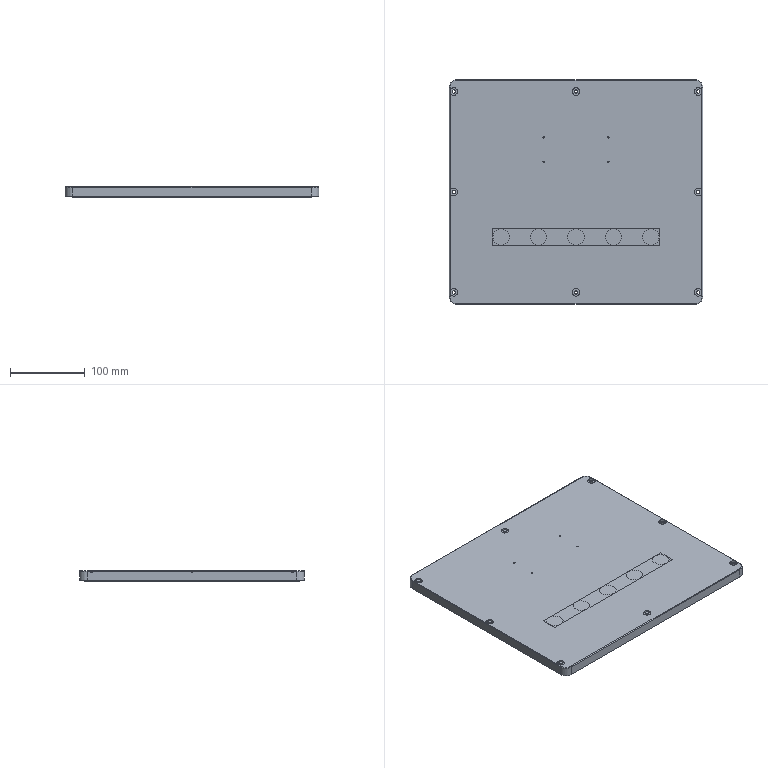NC program | NX | posted with a generic post | part box 338 x 300 x 14.5 mm
Lines 1 to 2036 of 2954, first 1954 of 2022 lines:
N10 G17 G21 G94 G90
(FLOOR_WALL , TOOL : D63)
N12 T03 M6
N14 G54
N16 G17 G0 G90 X-207. Y153.497 S6500 M3
N18 G43 Z30. H3
N20 Z3.
N22 G94 G1 Z0. F1250.
N24 X-204.
N26 X204.
N28 Y106.531
N30 X-204.
N32 Y59.565
N34 X204.
N36 Y12.599
N38 X-204.
N40 Y-34.368
N42 X204.
N44 Y-81.334
N46 X-204.
N48 Y-128.3
N50 X204.
N52 X207.
N54 Z3.
N56 G0 Z30.
N58 M5
(DRILLING_COPY_1 , TOOL : D6A45)
N60 T01 M6
N62 G54
N64 G17 G0 G90 X163. Y-134. S5000 M3
N66 G43 Z30. H1
N68 G94 G81 G98 Z-0.6 F250. R3.
N70 X100. Y-60.
N72 X163. Y0.
N74 Y134.
N76 X0.
N78 X-43. Y73.
N80 Y40.
N82 X43. Y73.
N84 Y40.
N86 X50. Y-60.
N88 X0.
N90 Y-134.
N92 X-50. Y-60.
N94 X-100.
N96 X-163. Y-134.
N98 Y0.
N100 Y134.
N102 G80
N104 G0 X-163. Y134. Z30.
N106 M5
(DRILLING_COPY_COPY , TOOL : 2.1ZT)
N108 T20 M6
N110 G54
N112 G17 G0 G90 X43. Y73. S1447 M3
N114 G43 Z30. H20
N116 G94 G83 G98 Z-7.116 F100. Q2. R3.
N118 Y40.
N120 X-43.
N122 Y73.
N124 G80
N126 G0 X-43. Y73. Z30.
N128 M5
(DRILLING_COPY_COPY_COPY , TOOL : 4.5ZT)
N130 T11 M6
N132 G54
N134 G17 G0 G90 X-163. Y134. S1447 M3
N136 G43 Z30. H11
N138 G94 G83 G98 Z-15.352 F100. Q2. R3.
N140 Y0.
N142 Y-134.
N144 X0.
N146 X163.
N148 Y0.
N150 Y134.
N152 X0.
N154 G80
N156 G0 X0. Y134. Z30.
N158 M5
(ADAPTIVE_MILLING , TOOL : D10)
N160 T04 M6
N162 G54
N164 G17 G0 G90 X-180.209 Y-0.062 S9500 M3
N166 G43 Z30. H4
N168 Z-13.5
N170 G94 G1 Z-14.5 F1000.
N172 X-179.429 Y-0.342 F3000.
N174 X-178.64 Y-0.598
N176 G3 X-177.562 Y-0.062 R1.017
N178 X-176.801 Y3.001 R8.28
N180 X-176.519 Y12.869 R111.643
N182 G1 X-176.514 Y15.119
N184 X-176.511 Y18.994
N186 X-176.51 Y32.619
N188 Y150.369
N190 Y150.494
N192 X-176.508 Y150.619
N194 G2 X-174.014 Y154.9 R5.714
N196 X-168.574 Y156.964 R12.307
N198 X-160.721 Y157.449 R56.36
N200 G1 X-159.721 Y157.46
N202 X-158.471 Y157.47
N204 X-156.846 Y157.478
N206 X-154.846 Y157.483
N208 X-151.596 Y157.487
N210 X-143.596 Y157.488
N212 X-29.346
N214 X-28.596 Y157.492
N216 X-27.471 Y157.494
N218 X-26.596
N220 X-25.846 Y157.496
N222 X-24.721
N224 X-24.346 Y157.495
N226 X-23.471 Y157.498
N228 X-22.471 Y157.496
N230 X-21.971
N232 X-21.346 Y157.497
N234 X-19.971
N236 X-19.221 Y157.496
N238 X-18.221 Y157.499
N240 X-16.971 Y157.497
N242 X-16.221 Y157.498
N244 X-15.221
N246 X-14.846 Y157.497
N248 X-13.596 Y157.5
N250 X-12.721 Y157.498
N252 X-11.471 Y157.5
N254 X-10.096 Y157.497
N256 X-9.471 Y157.499
N258 X-7.971 Y157.498
N260 X-6.971 Y157.496
N262 X-6.096 Y157.499
N264 X-5.471 Y157.498
N266 X-4.721 Y157.496
N268 X-3.846 Y157.499
N270 X-3.221 Y157.498
N272 X-2.471 Y157.497
N274 X-1.596 Y157.499
N276 X-0.971 Y157.498
N278 X-0.221 Y157.497
N280 X0.654 Y157.499
N282 X1.279 Y157.498
N284 X2.029 Y157.497
N286 X2.904 Y157.499
N288 X3.529 Y157.498
N290 X4.279 Y157.497
N292 X5.279 Y157.499
N294 X6.029 Y157.498
N296 X7.154 Y157.5
N298 X7.654 Y157.501
N300 X8.904 Y157.498
N302 X9.529 Y157.499
N304 X11.029 Y157.498
N306 X11.654 Y157.497
N308 X12.654 Y157.499
N310 X13.904 Y157.497
N312 X14.654 Y157.499
N314 X15.529 Y157.498
N316 X16.154 Y157.497
N318 X17.529 Y157.5
N320 X18.904 Y157.497
N322 X20.029 Y157.5
N324 X20.779 Y157.499
N326 X22.029 Y157.5
N328 X23.029 Y157.498
N330 X24.154 Y157.501
N332 X25.404 Y157.498
N334 X26.029 Y157.499
N336 X27.529 Y157.498
N338 X28.154 Y157.497
N340 X29.154 Y157.499
N342 X30.529 Y157.497
N344 X31.154 Y157.498
N346 X32.654 Y157.497
N348 X33.279 Y157.496
N350 X34.404 Y157.499
N352 X35.529 Y157.497
N354 X36.529 Y157.5
N356 X37.779 Y157.497
N358 X38.529 Y157.499
N360 X39.404 Y157.498
N362 X40.029 Y157.497
N364 X40.779 Y157.498
N366 X41.904
N368 X42.404 Y157.497
N370 X43.154 Y157.498
N372 X44.279 Y157.497
N374 X44.654
N376 X45.529 Y157.499
N378 X46.529 Y157.497
N380 X47.029 Y157.496
N382 X47.779 Y157.498
N384 X48.779
N386 X49.279 Y157.497
N388 X50.154 Y157.499
N390 X51.279 Y157.497
N392 X52.654 Y157.5
N394 X53.279 Y157.499
N396 X54.779 Y157.5
N398 X55.404 Y157.501
N400 X56.529 Y157.499
N402 X57.529 Y157.501
N404 X58.279 Y157.499
N406 X59.404 Y157.5
N408 X59.779 Y157.501
N410 X60.779 Y157.499
N412 X61.529 Y157.5
N414 X62.529 Y157.499
N416 X63.154 Y157.497
N418 X64.279 Y157.5
N420 X65.279 Y157.498
N422 X66.654 Y157.501
N424 X67.904 Y157.498
N426 X69.154 Y157.501
N428 X70.404 Y157.498
N430 X71.029 Y157.499
N432 X72.529 Y157.498
N434 X73.529 Y157.496
N436 X74.279 Y157.498
N438 X75.279 Y157.497
N440 X76.029 Y157.498
N442 X76.529 Y157.499
N444 X77.654 Y157.497
N446 X78.779 Y157.5
N448 X79.779 Y157.498
N450 X80.529 Y157.499
N452 X81.654 Y157.498
N454 X82.029
N456 X83.029 Y157.5
N458 X83.779 Y157.498
N460 X84.904 Y157.5
N462 X85.529
N464 X86.529 Y157.497
N466 X87.154 Y157.499
N468 X88.654 Y157.498
N470 X89.279 Y157.497
N472 X90.404 Y157.5
N474 X91.403 Y157.498
N476 X92.778 Y157.501
N478 X94.028 Y157.498
N480 X95.278 Y157.501
N482 X96.528 Y157.498
N484 X97.903 Y157.501
N486 X99.028 Y157.498
N488 X99.778 Y157.5
N490 X100.778 Y157.498
N492 X101.153
N494 X102.403 Y157.5
N496 X103.278 Y157.499
N498 X104.653 Y157.501
N500 X105.528 Y157.499
N502 X106.778 Y157.501
N504 X108.028 Y157.498
N506 X108.653 Y157.499
N508 X110.153 Y157.498
N510 X110.778 Y157.497
N512 X111.778 Y157.499
N514 X113.028 Y157.497
N516 X113.778 Y157.499
N518 X114.778 Y157.498
N520 X115.528
N522 X116.028 Y157.499
N524 X117.028 Y157.498
N526 X117.778 Y157.499
N528 X118.903 Y157.498
N530 X119.528
N532 X120.528 Y157.501
N534 X121.278 Y157.499
N536 X122.278 Y157.5
N538 X122.778 Y157.501
N540 X123.528 Y157.499
N542 X124.653 Y157.501
N544 X125.278 Y157.5
N546 X126.153 Y157.498
N548 X127.153 Y157.5
N550 X127.903 Y157.499
N552 X129.028 Y157.5
N554 X129.653 Y157.501
N556 X130.528 Y157.499
N558 X131.153 Y157.5
N560 X131.903 Y157.501
N562 X132.778 Y157.499
N564 X133.403 Y157.5
N566 X134.153 Y157.502
N568 X135.028 Y157.499
N570 X136.278 Y157.501
N572 X137.528 Y157.498
N574 X138.278 Y157.5
N576 X139.278 Y157.498
N578 X139.653
N580 X140.903 Y157.5
N582 X141.778 Y157.498
N584 X143.153 Y157.501
N586 X144.153 Y157.499
N588 X144.903 Y157.5
N590 X146.028 Y157.498
N592 X146.403
N594 X147.653 Y157.501
N596 X148.653 Y157.498
N598 X149.403 Y157.5
N600 X150.528 Y157.498
N602 X150.903
N604 X152.028 Y157.5
N606 X153.278 Y157.497
N608 X154.028 Y157.499
N610 X155.028 Y157.498
N612 X155.528 Y157.497
N614 X156.278 Y157.499
N616 X157.403 Y157.497
N618 X158.028 Y157.498
N620 X158.903 Y157.5
N622 X159.903 Y157.498
N624 X160.653 Y157.499
N626 X161.778 Y157.498
N628 X162.403 Y157.497
N630 X163.278 Y157.499
N632 X163.903 Y157.498
N634 X164.653 Y157.497
N636 X165.528 Y157.499
N638 X166.153 Y157.498
N640 X166.903 Y157.497
N642 X167.778 Y157.499
N644 X168.403 Y157.498
N646 G2 X171.116 Y157.192 R7.132
N648 X174.868 Y153.36 R7.122
N650 X176.232 Y147.293 R18.07
N652 X176.483 Y135.799 R164.122
N654 G1 X176.487 Y132.549
N656 X176.489 Y124.674
N658 Y-150.576
N660 X176.484 Y-150.701
N662 X176.477 Y-150.826
N664 X176.465 Y-150.95
N666 G2 X173.623 Y-155.167 R6.027
N668 X167.856 Y-157.069 R13.655
N670 X158.87 Y-157.468 R78.215
N672 G1 X157.495 Y-157.476
N674 X155.62 Y-157.482
N676 X152.87 Y-157.486
N678 X147.37 Y-157.488
N680 X-169.505
N682 X-169.63 Y-157.486
N684 G2 X-173.832 Y-155.083 R5.703
N686 X-175.984 Y-149.417 R12.271
N688 X-176.456 Y-141.187 R61.689
N690 G1 X-176.465 Y-140.187
N692 X-176.474 Y-138.812
N694 X-176.48 Y-137.187
N696 X-176.485 Y-134.937
N698 X-176.488 Y-130.937
N700 X-176.489 Y-115.562
N702 Y-56.062
N704 X-176.492 Y-55.437
N706 X-176.495 Y-53.687
N708 X-176.494 Y-52.062
N710 Y-51.687
N712 X-176.496 Y-51.062
N714 Y-49.812
N716 Y-49.187
N718 X-176.499 Y-48.187
N720 X-176.496 Y-46.937
N722 X-176.5 Y-45.687
N724 X-176.497 Y-44.312
N726 X-176.5 Y-43.312
N728 X-176.498 Y-42.187
N730 X-176.5 Y-41.312
N732 X-176.499 Y-40.687
N734 X-176.497 Y-39.937
N736 X-176.5 Y-38.937
N738 X-176.499 Y-38.187
N740 X-176.5 Y-37.062
N742 X-176.501 Y-36.562
N744 X-176.499 Y-35.437
N746 X-176.5 Y-34.562
N748 X-176.498 Y-33.437
N750 X-176.5 Y-32.562
N752 X-176.498 Y-31.187
N754 X-176.5 Y-30.187
N756 X-176.498 Y-28.937
N758 X-176.499 Y-28.187
N760 Y-27.312
N762 X-176.498 Y-26.812
N764 X-176.5 Y-25.937
N766 X-176.498 Y-24.687
N768 X-176.501 Y-23.312
N770 X-176.5 Y-22.687
N772 Y-21.187
N774 X-176.502 Y-20.312
N776 X-176.499 Y-19.312
N778 X-176.502 Y-18.062
N780 X-176.5 Y-17.187
N782 X-176.501 Y-16.187
N784 X-176.502 Y-15.812
N786 X-176.499 Y-14.812
N788 X-176.502 Y-13.562
N790 X-176.5 Y-12.937
N792 X-176.501 Y-11.438
N794 X-176.502 Y-10.688
N796 X-176.5 Y-9.688
N798 X-176.502 Y-8.438
N800 X-176.5 Y-7.688
N802 X-176.501 Y-6.688
N804 X-176.502 Y-6.313
N806 X-176.499 Y-5.063
N808 X-176.501 Y-4.188
N810 X-176.5 Y-3.813
N812 X-176.499 Y-3.688
N814 X-176.497 Y-3.563
N816 X-176.489 Y-3.313
N818 X-176.484 Y-3.188
N820 X-176.477 Y-3.063
N822 G2 X-175.845 Y3.028 R826.011
N824 G3 X-175.53 Y15.897 R182.279
N826 G1 X-175.525 Y18.397
N828 X-175.522 Y22.772
N830 X-175.521 Y38.022
N832 Y147.397
N834 X-175.519 Y147.522
N836 X-175.517 Y147.647
N838 G2 X-171.822 Y153.83 R7.666
N840 X-165.599 Y155.948 R15.428
N842 X-156.744 Y156.439 R69.654
N844 G1 X-155.494 Y156.452
N846 X-154.244 Y156.46
N848 X-152.619 Y156.467
N850 X-150.369 Y156.473
N852 X-146.744 Y156.476
N854 X-137.619 Y156.477
N856 X-32.369 Y156.478
N858 X-31.494 Y156.482
N860 X-30.369 Y156.485
N862 X-29.494
N864 X-28.744 Y156.489
N866 X-27.619 Y156.49
N868 X-26.619
N870 X-25.869 Y156.493
N872 X-24.869
N874 X-24.369
N876 X-23.494 Y156.495
N878 X-22.494 Y156.494
N880 X-22.119
N882 X-21.119 Y156.496
N884 X-20.119 Y156.495
N886 X-19.744
N888 X-18.369 Y156.498
N890 X-17.369 Y156.496
N892 X-16.119 Y156.5
N894 X-15.369 Y156.498
N896 X-14.119 Y156.5
N898 X-13.619
N900 X-12.869 Y156.499
N902 X-11.744
N904 X-11.244 Y156.5
N906 X-9.744 Y156.496
N908 X-8.869 Y156.498
N910 X-7.619 Y156.497
N912 X-6.994 Y156.496
N914 X-5.994 Y156.499
N916 X-5.244 Y156.497
N918 X-3.994 Y156.498
N920 X-3.619 Y156.499
N922 X-2.744 Y156.497
N924 X-1.744 Y156.499
N926 X-0.744 Y156.497
N928 X0.256 Y156.498
N930 X1.381 Y156.496
N932 X2.631 Y156.499
N934 X3.631 Y156.497
N936 X4.881 Y156.5
N938 X6.256 Y156.497
N940 X7.256 Y156.499
N942 X8.631 Y156.496
N944 X9.881 Y156.499
N946 X11.131 Y156.496
N948 X12.381 Y156.499
N950 X13.506 Y156.497
N952 X14.631 Y156.499
N954 X16.006 Y156.497
N956 X17.381 Y156.5
N958 X18.506 Y156.498
N960 X19.256 Y156.499
N962 X20.506 Y156.498
N964 X21.131 Y156.497
N966 X21.756 Y156.499
N968 X23.006 Y156.498
N970 X23.631 Y156.497
N972 X24.506 Y156.499
N974 X25.506 Y156.497
N976 X26.631 Y156.499
N978 X27.631 Y156.498
N980 X28.631 Y156.499
N982 X29.256
N984 X30.131 Y156.496
N986 X31.506 Y156.5
N988 X32.756 Y156.497
N990 X33.756 Y156.499
N992 X34.381 Y156.498
N994 X35.131 Y156.496
N996 X35.881 Y156.498
N998 X37.131 Y156.497
N1000 X37.631 Y156.496
N1002 X38.506 Y156.498
N1004 X39.256 Y156.497
N1006 X39.881 Y156.496
N1008 X40.881 Y156.498
N1010 X41.881 Y156.497
N1012 X42.756 Y156.498
N1014 X43.131 Y156.499
N1016 X44.131 Y156.497
N1018 X45.381 Y156.499
N1020 X46.381 Y156.497
N1022 X47.506 Y156.499
N1024 X48.381 Y156.498
N1026 X49.381 Y156.499
N1028 X49.756 Y156.5
N1030 X51.006 Y156.498
N1032 X52.006 Y156.5
N1034 X53.631 Y156.497
N1036 X54.756 Y156.5
N1038 X55.631 Y156.499
N1040 X56.631 Y156.5
N1042 X57.131 Y156.501
N1044 X58.131 Y156.499
N1046 X59.006 Y156.5
N1048 X60.006 Y156.499
N1050 X60.381 Y156.498
N1052 X61.631 Y156.5
N1054 X62.631 Y156.498
N1056 X63.256 Y156.499
N1058 X63.881 Y156.501
N1060 X64.881 Y156.499
N1062 X65.631 Y156.5
N1064 X66.381 Y156.502
N1066 X67.631 Y156.498
N1068 X68.506 Y156.5
N1070 X69.506 Y156.498
N1072 X69.881 Y156.497
N1074 X71.381 Y156.5
N1076 X72.006 Y156.499
N1078 X73.506 Y156.5
N1080 X74.131 Y156.501
N1082 X74.881 Y156.499
N1084 X76.006 Y156.5
N1086 X76.631 Y156.501
N1088 X77.506 Y156.499
N1090 X78.506 Y156.5
N1092 X79.631 Y156.498
N1094 X80.756 Y156.5
N1096 X81.506 Y156.498
N1098 X82.381 Y156.5
N1100 X82.881 Y156.501
N1102 X83.756 Y156.499
N1104 X84.756 Y156.5
N1106 X85.131
N1108 X86.256 Y156.498
N1110 X86.881
N1112 X87.631 Y156.5
N1114 X88.631 Y156.498
N1116 X89.631 Y156.5
N1118 X90.256
N1120 X91.131 Y156.498
N1122 X92.131 Y156.5
N1124 X92.631 Y156.501
N1126 X93.506 Y156.5
N1128 X94.756
N1130 X95.506 Y156.501
N1132 X96.506 Y156.499
N1134 X97.756 Y156.501
N1136 X98.756 Y156.499
N1138 X99.881 Y156.501
N1140 X100.756 Y156.499
N1142 X101.756 Y156.501
N1144 X102.381 Y156.5
N1146 X102.881 Y156.499
N1148 X103.756 Y156.501
N1150 X104.131
N1152 X105.381 Y156.498
N1154 X106.631 Y156.501
N1156 X108.006 Y156.497
N1158 X109.256 Y156.5
N1160 X110.381 Y156.497
N1162 X111.131 Y156.498
N1164 X112.381 Y156.497
N1166 X112.881
N1168 X113.756 Y156.499
N1170 X114.631 Y156.497
N1172 X115.756 Y156.499
N1174 X116.756 Y156.497
N1176 X118.006 Y156.5
N1178 X119.131 Y156.498
N1180 X120.256 Y156.501
N1182 X121.506 Y156.498
N1184 X122.381 Y156.5
N1186 X123.131 Y156.499
N1188 X123.631 Y156.498
N1190 X124.881 Y156.501
N1192 X125.631 Y156.499
N1194 X126.631 Y156.5
N1196 X127.006 Y156.501
N1198 X128.256 Y156.499
N1200 X129.256 Y156.501
N1202 X130.631 Y156.498
N1204 X131.506 Y156.5
N1206 X132.631 Y156.499
N1208 X133.756 Y156.501
N1210 X134.756 Y156.499
N1212 X135.756 Y156.5
N1214 X136.131 Y156.501
N1216 X137.255 Y156.498
N1218 X138.255 Y156.5
N1220 X139.13 Y156.499
N1222 X140.13 Y156.5
N1224 X140.505 Y156.501
N1226 X141.505 Y156.499
N1228 X142.38 Y156.5
N1230 X143.505 Y156.499
N1232 X144.505 Y156.5
N1234 X145.13
N1236 X146.005 Y156.498
N1238 X147.005 Y156.5
N1240 X148.255 Y156.497
N1242 X149.255 Y156.5
N1244 X149.88 Y156.499
N1246 X150.505 Y156.497
N1248 X151.63 Y156.5
N1250 X152.755 Y156.497
N1252 X153.88 Y156.499
N1254 G2 X167.129 Y156.463 R678.019
N1256 X172.891 Y152.714 R7.73
N1258 X174.981 Y146.35 R15.787
N1260 X175.451 Y136.618 R79.987
N1262 G1 X175.459 Y135.493
N1264 X175.467 Y133.868
N1266 X175.472 Y131.743
N1268 X175.476 Y128.368
N1270 X175.478 Y120.868
N1272 Y63.118
N1274 X175.482 Y62.368
N1276 X175.483 Y61.243
N1278 Y60.368
N1280 X175.486 Y59.618
N1282 X175.485 Y58.493
N1284 Y58.118
N1286 X175.487 Y57.243
N1288 X175.486 Y56.243
N1290 X175.485 Y55.743
N1292 X175.487 Y55.118
N1294 Y53.743
N1296 X175.486 Y53.118
N1298 X175.488 Y52.118
N1300 X175.486 Y50.743
N1302 X175.489 Y49.743
N1304 X175.486 Y48.618
N1306 X175.489 Y47.618
N1308 X175.488 Y46.868
N1310 X175.489 Y45.743
N1312 X175.49 Y45.243
N1314 X175.488 Y44.118
N1316 X175.49 Y43.118
N1318 X175.487 Y41.868
N1320 X175.489 Y41.118
N1322 X175.488 Y40.243
N1324 X175.487 Y39.743
N1326 X175.489 Y38.743
N1328 X175.488 Y37.868
N1330 X175.49 Y36.368
N1332 X175.489 Y35.618
N1334 X175.49 Y34.618
N1336 X175.489 Y33.993
N1338 X175.488 Y33.493
N1340 X175.49 Y32.493
N1342 X175.487 Y31.243
N1344 X175.49 Y30.243
N1346 X175.487 Y28.993
N1348 X175.489 Y28.243
N1350 X175.488 Y27.368
N1352 X175.487 Y26.868
N1354 X175.489 Y25.868
N1356 X175.488 Y24.993
N1358 X175.49 Y23.493
N1360 X175.489 Y22.743
N1362 X175.49 Y21.868
N1364 X175.491 Y21.243
N1366 X175.487 Y19.868
N1368 X175.49 Y18.618
N1370 X175.488 Y17.493
N1372 X175.489 Y16.868
N1374 X175.488 Y15.493
N1376 X175.486 Y14.618
N1378 X175.488 Y13.868
N1380 X175.487 Y12.868
N1382 X175.486 Y12.368
N1384 X175.488 Y11.493
N1386 X175.487 Y10.368
N1388 X175.49 Y8.993
N1390 X175.489 Y8.368
N1392 X175.49 Y6.868
N1394 X175.492 Y5.993
N1396 X175.49 Y5.243
N1398 Y4.243
N1400 X175.491 Y3.743
N1402 X175.49 Y2.993
N1404 X175.491 Y1.868
N1406 X175.49 Y1.243
N1408 X175.488 Y0.368
N1410 X175.49 Y-0.507
N1412 X175.487 Y-1.757
N1414 X175.49 Y-3.007
N1416 X175.489 Y-3.632
N1418 X175.49 Y-5.132
N1420 X175.491 Y-5.882
N1422 X175.489 Y-6.632
N1424 X175.49 Y-7.507
N1426 X175.491 Y-8.007
N1428 X175.489 Y-9.007
N1430 X175.49 Y-9.882
N1432 X175.487 Y-11.257
N1434 X175.49 Y-12.257
N1436 X175.487 Y-13.507
N1438 X175.489 Y-14.382
N1440 X175.487 Y-15.632
N1442 X175.489 Y-16.382
N1444 X175.487 Y-17.507
N1446 Y-17.882
N1448 X175.489 Y-18.757
N1450 X175.486 Y-20.132
N1452 X175.489 Y-21.007
N1454 X175.487 Y-22.257
N1456 X175.49 Y-23.507
N1458 X175.488 Y-24.132
N1460 X175.49 Y-25.632
N1462 X175.491 Y-26.257
N1464 X175.488 Y-27.257
N1466 X175.491 Y-28.507
N1468 X175.489 Y-29.257
N1470 X175.49 Y-30.257
N1472 X175.489 Y-31.007
N1474 X175.488 Y-31.507
N1476 X175.49 Y-32.507
N1478 X175.489 Y-33.257
N1480 X175.49 Y-34.257
N1482 X175.491 Y-34.882
N1484 X175.488 Y-35.882
N1486 X175.491 Y-37.132
N1488 X175.489 Y-37.882
N1490 X175.49 Y-38.757
N1492 X175.491 Y-39.257
N1494 X175.489 Y-40.132
N1496 X175.491 Y-41.382
N1498 X175.488 Y-42.632
N1500 X175.489 Y-43.257
N1502 X175.488 Y-44.757
N1504 X175.486 Y-45.382
N1506 X175.489 Y-46.257
N1508 X175.487 Y-47.382
N1510 X175.489 Y-48.257
N1512 X175.487 Y-49.632
N1514 X175.489 Y-50.507
N1516 X175.487 Y-51.632
N1518 X175.489 Y-52.507
N1520 X175.487 Y-53.507
N1522 X175.486 Y-54.007
N1524 X175.488 Y-54.757
N1526 X175.487 Y-55.757
N1528 X175.488 Y-56.382
N1530 X175.489 Y-56.882
N1532 X175.487 Y-57.882
N1534 X175.49 Y-59.257
N1536 X175.489 Y-59.882
N1538 X175.49 Y-61.382
N1540 X175.491 Y-62.007
N1542 X175.488 Y-63.007
N1544 X175.491 Y-64.382
N1546 X175.488 Y-65.507
N1548 X175.49 Y-66.257
N1550 X175.488 Y-67.507
N1552 X175.49 Y-68.507
N1554 X175.488 Y-69.507
N1556 X175.489 Y-70.257
N1558 X175.487 Y-71.382
N1560 X175.488 Y-72.007
N1562 X175.49 Y-73.007
N1564 X175.489 Y-73.632
N1566 X175.49 Y-75.132
N1568 X175.491 Y-75.882
N1570 X175.49 Y-76.632
N1572 Y-77.507
N1574 X175.491 Y-78.007
N1576 X175.489 Y-79.007
N1578 X175.49 Y-79.882
N1580 X175.487 Y-81.257
N1582 X175.49 Y-82.257
N1584 X175.487 Y-83.632
N1586 X175.49 Y-84.882
N1588 X175.489 Y-85.507
N1590 X175.49 Y-87.007
N1592 X175.491 Y-87.882
N1594 X175.489 Y-88.757
N1596 X175.491 Y-90.007
N1598 X175.488 Y-91.257
N1600 X175.489 Y-92.007
N1602 X175.488 Y-93.007
N1604 X175.487 Y-93.382
N1606 X175.49 Y-94.632
N1608 X175.488 Y-95.507
N1610 X175.49 Y-96.757
N1612 X175.487 Y-98.007
N1614 X175.489 Y-98.632
N1616 X175.487 Y-100.132
N1618 X175.486 Y-100.757
N1620 X175.488 Y-101.632
N1622 X175.487 Y-102.757
N1624 X175.489 Y-103.632
N1626 X175.487 Y-105.007
N1628 X175.489 Y-105.882
N1630 X175.487 Y-107.007
N1632 X175.489 Y-107.882
N1634 X175.487 Y-108.882
N1636 X175.486 Y-109.382
N1638 X175.488 Y-110.132
N1640 X175.487 Y-111.132
N1642 X175.488 Y-111.757
N1644 X175.489 Y-112.257
N1646 X175.487 Y-113.382
N1648 X175.49 Y-114.632
N1650 X175.488 Y-115.507
N1652 X175.491 Y-116.882
N1654 X175.488 Y-117.882
N1656 X175.491 Y-119.132
N1658 X175.489 Y-119.882
N1660 X175.49 Y-120.882
N1662 X175.489 Y-121.632
N1664 X175.488 Y-122.132
N1666 X175.49 Y-123.132
N1668 X175.489 Y-123.882
N1670 X175.49 Y-125.007
N1672 Y-125.632
N1674 X175.488 Y-126.507
N1676 X175.489 Y-127.257
N1678 X175.488 Y-128.132
N1680 X175.487 Y-128.507
N1682 X175.49 Y-129.882
N1684 X175.489 Y-130.507
N1686 X175.49 Y-132.007
N1688 X175.491 Y-132.632
N1690 X175.488 Y-133.757
N1692 X175.49 Y-134.757
N1694 X175.487 Y-136.007
N1696 X175.488 Y-136.632
N1698 X175.487 Y-138.132
N1700 X175.486 Y-138.882
N1702 X175.488 Y-139.632
N1704 X175.487 Y-140.507
N1706 X175.486 Y-141.007
N1708 X175.489 Y-142.007
N1710 X175.487 Y-142.882
N1712 X175.49 Y-144.382
N1714 X175.489 Y-145.132
N1716 X175.49 Y-146.007
N1718 Y-146.507
N1720 G2 X174.68 Y-150.751 R8.308
N1722 X169.816 Y-154.858 R9.247
N1724 X163.104 Y-156.217 R22.548
N1726 X151.734 Y-156.47 R179.365
N1728 G1 X148.984 Y-156.474
N1730 X144.109 Y-156.477
N1732 X98.734 Y-156.478
N1734 X-166.391
N1736 X-166.641 Y-156.475
N1738 X-166.765 Y-156.471
N1740 G2 X-172.829 Y-152.794 R7.645
N1742 X-174.948 Y-146.572 R15.398
N1744 X-175.446 Y-137.217 R73.377
N1746 G1 X-175.456 Y-135.967
N1748 X-175.464 Y-134.467
N1750 X-175.471 Y-132.467
N1752 X-175.475 Y-129.842
N1754 X-175.477 Y-124.842
N1756 X-175.478 Y-71.967
N1758 Y-59.092
N1760 X-175.482 Y-58.217
N1762 X-175.486 Y-56.717
N1764 X-175.487 Y-55.217
N1766 Y-54.592
N1768 X-175.491 Y-53.717
N1770 Y-52.967
N1772 X-175.49 Y-51.967
N1774 X-175.494 Y-51.092
N1776 Y-50.217
N1778 X-175.493 Y-49.717
N1780 X-175.497 Y-48.467
N1782 X-175.496 Y-47.467
N1784 Y-46.842
N1786 X-175.498 Y-46.092
N1788 X-175.496 Y-44.967
N1790 X-175.498 Y-44.092
N1792 X-175.497 Y-43.092
N1794 Y-42.717
N1796 X-175.499 Y-41.592
N1798 X-175.497 Y-40.342
N1800 X-175.499 Y-39.467
N1802 Y-38.592
N1804 X-175.498 Y-38.092
N1806 X-175.499 Y-37.217
N1808 X-175.498 Y-36.342
N1810 X-175.497 Y-35.842
N1812 X-175.5 Y-34.717
N1814 X-175.498 Y-33.842
N1816 X-175.5 Y-32.592
N1818 X-175.497 Y-31.342
N1820 X-175.499 Y-30.592
N1822 X-175.498 Y-29.467
N1824 X-175.497 Y-28.967
N1826 X-175.499 Y-27.967
N1828 X-175.497 Y-26.967
N1830 X-175.5 Y-25.967
N1832 X-175.498 Y-24.967
N1834 X-175.501 Y-23.842
N1836 X-175.498 Y-22.217
N1838 X-175.502 Y-20.842
N1840 X-175.5 Y-19.967
N1842 X-175.501 Y-18.717
N1844 X-175.502 Y-18.092
N1846 X-175.5 Y-17.217
N1848 X-175.502 Y-16.217
N1850 X-175.501 Y-15.592
N1852 X-175.499 Y-14.717
N1854 X-175.501 Y-13.967
N1856 X-175.5 Y-12.717
N1858 X-175.499 Y-12.092
N1860 X-175.501 Y-11.217
N1862 X-175.499 Y-10.217
N1864 Y-9.842
N1866 X-175.501 Y-8.842
N1868 X-175.499 Y-7.842
N1870 G2 X-175.061 Y0.516 R72.626
N1872 G3 X-174.548 Y15.753 R179.007
N1874 G1 X-174.541 Y17.878
N1876 X-174.536 Y20.628
N1878 X-174.533 Y25.128
N1880 X-174.532 Y38.628
N1882 Y144.378
N1884 X-174.53 Y144.753
N1886 G2 X-169.734 Y152.945 R9.001
N1888 X-162.952 Y154.976 R18.242
N1890 X-152.968 Y155.437 R91.025
N1892 G1 X-151.593 Y155.447
N1894 X-149.843 Y155.455
N1896 X-147.843 Y155.46
N1898 X-144.593 Y155.464
N1900 X-138.093 Y155.466
N1902 X-35.343 Y155.467
N1904 X-34.218 Y155.473
N1906 X-33.218 Y155.474
N1908 X-32.343 Y155.475
N1910 X-31.468 Y155.48
N1912 X-30.718 Y155.481
N1914 X-29.468
N1916 X-28.593 Y155.486
N1918 X-27.718 Y155.487
N1920 X-27.218
N1922 X-26.218 Y155.49
N1924 X-25.218
N1926 X-24.718 Y155.489
N1928 X-23.593 Y155.493
N1930 X-22.468 Y155.492
N1932 X-21.093 Y155.496
N1934 X-19.968 Y155.494
N1936 X-18.968 Y155.497
N1938 X-17.968 Y155.496
N1940 X-17.343 Y155.495
N1942 X-16.593 Y155.497
N1944 X-15.343 Y155.498
N1946 X-14.468 Y155.496
N1948 X-13.593 Y155.499
N1950 X-12.843 Y155.498
N1952 X-12.218 Y155.496
N1954 X-11.093 Y155.499
N1956 X-9.968 Y155.496
N1958 X-8.718 Y155.499
N1960 X-7.718 Y155.497
N1962 X-6.343 Y155.5
N1964 X-5.218 Y155.497
N1966 X-4.093 Y155.499
N1968 X-3.093 Y155.497
N1970 X-2.343 Y155.498
N1972 X-1.218 Y155.497
N1974 X-0.718 Y155.496
N1976 X0.282 Y155.498
N1978 X1.407 Y155.496
N1980 X2.407 Y155.499
N1982 X3.032 Y155.498
N1984 X3.782 Y155.496
N1986 X4.657 Y155.498
N1988 X5.657 Y155.497
N1990 X6.032 Y155.496
N1992 X7.032 Y155.498
N1994 X8.032 Y155.497
N1996 X8.532 Y155.496
N1998 X9.657 Y155.498
N2000 X10.907 Y155.496
N2002 X12.032 Y155.499
N2004 X13.282 Y155.496
N2006 X14.531 Y155.499
N2008 X15.781 Y155.497
N2010 X16.906 Y155.5
N2012 X18.156 Y155.497
N2014 X19.281 Y155.499
N2016 X20.406 Y155.497
N2018 X21.531 Y155.499
N2020 X22.781 Y155.497
N2022 X23.781 Y155.499
N2024 X24.406 Y155.498
N2026 X25.031 Y155.497
N2028 X26.156 Y155.499
N2030 X27.531 Y155.496
N2032 X28.781 Y155.499
N2034 X30.031 Y155.497
N2036 X31.031 Y155.499
N2038 X31.656 Y155.498
N2040 X32.406 Y155.496
N2042 X33.156 Y155.497
N2044 X34.406 Y155.496
N2046 X35.031 Y155.495
N2048 X36.031 Y155.498
N2050 X37.156 Y155.495
N2052 X38.281 Y155.498
N2054 X39.156 Y155.497
N2056 X40.156 Y155.498
N2058 X40.531 Y155.499
N2060 X41.656 Y155.497
N2062 X42.656 Y155.498
N2064 X43.656 Y155.497
N2066 X44.281
N2068 X45.156 Y155.499
N2070 X46.406 Y155.496
N2072 X47.406 Y155.499
N2074 X48.531 Y155.497
N2076 X49.406 Y155.499
N2078 X50.281 Y155.498
N2080 X50.781 Y155.497
N2082 X51.781 Y155.499
N2084 X52.156 Y155.5
N2086 X53.156 Y155.498
N2088 X54.156 Y155.5
N2090 X55.156 Y155.499
N2092 X56.406 Y155.501
N2094 X57.781 Y155.498
N2096 X58.656 Y155.5
N2098 X59.656 Y155.498
N2100 X60.406 Y155.499
N2102 X61.281 Y155.501
N2104 X62.406 Y155.499
N2106 X63.781 Y155.502
N2108 X64.781 Y155.499
N2110 X65.406 Y155.5
N2112 X66.156 Y155.502
N2114 X67.031 Y155.499
N2116 X68.031 Y155.5
N2118 X68.656 Y155.501
N2120 X69.656 Y155.499
N2122 X71.156 Y155.502
N2124 X72.531 Y155.498
N2126 X73.656 Y155.501
N2128 X74.781 Y155.499
N2130 X76.031 Y155.501
N2132 X76.906 Y155.499
N2134 X77.906 Y155.5
N2136 X78.656
N2138 X79.406 Y155.498
N2140 X80.281 Y155.5
N2142 X81.281 Y155.498
N2144 X81.656
N2146 X82.656 Y155.5
N2148 X83.656 Y155.498
N2150 X84.656 Y155.5
N2152 X85.031 Y155.501
N2154 X86.031 Y155.498
N2156 X87.031 Y155.5
N2158 X88.281 Y155.499
N2160 X89.156 Y155.5
N2162 X89.781 Y155.502
N2164 X91.031 Y155.499
N2166 X92.406 Y155.502
N2168 X93.781 Y155.498
N2170 X95.031 Y155.502
N2172 X95.906 Y155.5
N2174 X96.906 Y155.501
N2176 X97.406 Y155.502
N2178 X98.531 Y155.499
N2180 X99.406 Y155.501
N2182 X100.406 Y155.499
N2184 X101.031 Y155.5
N2186 X101.906 Y155.502
N2188 X103.031 Y155.499
N2190 X103.781 Y155.5
N2192 X105.031 Y155.499
N2194 X105.781 Y155.498
N2196 X106.656 Y155.499
N2198 X107.656 Y155.498
N2200 X108.031 Y155.497
N2202 X109.031 Y155.499
N2204 X110.281 Y155.496
N2206 X111.406 Y155.499
N2208 X112.281 Y155.497
N2210 X113.406 Y155.499
N2212 X114.406 Y155.497
N2214 X115.656 Y155.5
N2216 X116.781 Y155.497
N2218 X117.531 Y155.499
N2220 X118.781
N2222 X119.531 Y155.497
N2224 X120.281 Y155.499
N2226 X121.156 Y155.498
N2228 X121.531
N2230 X122.656 Y155.5
N2232 X123.531 Y155.499
N2234 X124.781 Y155.501
N2236 X125.656 Y155.499
N2238 X126.656 Y155.501
N2240 X127.281
N2242 X127.906 Y155.499
N2244 X129.156 Y155.501
N2246 X130.031 Y155.499
N2248 X131.281 Y155.501
N2250 X132.531 Y155.498
N2252 X133.406 Y155.5
N2254 X134.281 Y155.499
N2256 X134.656 Y155.498
N2258 X135.906 Y155.501
N2260 X136.781 Y155.499
N2262 X137.781 Y155.501
N2264 X138.406 Y155.5
N2266 X138.906 Y155.499
N2268 X140.031 Y155.501
N2270 X141.281 Y155.498
N2272 X142.281 Y155.501
N2274 X143.281 Y155.499
N2276 X144.656 Y155.501
N2278 X145.531 Y155.499
N2280 X146.781 Y155.5
N2282 X147.281 Y155.501
N2284 X148.031 Y155.499
N2286 X149.156 Y155.5
N2288 X149.531
N2290 X150.406 Y155.498
N2292 X151.531 Y155.5
N2294 X152.531 Y155.498
N2296 X153.531 Y155.5
N2298 X154.656 Y155.498
N2300 X155.656 Y155.5
N2302 X156.406 Y155.499
N2304 X157.031 Y155.497
N2306 X158.156 Y155.5
N2308 X159.281 Y155.497
N2310 X160.281 Y155.499
N2312 X161.281 Y155.497
N2314 X162.281 Y155.499
N2316 X162.656
N2318 G2 X166.862 Y155.056 R12.92
N2320 X172.255 Y150.135 R9.39
N2322 X174.078 Y143.031 R20.33
N2324 X174.451 Y131.792 R123.575
N2326 G1 X174.458 Y129.917
N2328 X174.463 Y127.292
N2330 X174.466 Y122.917
N2332 X174.467 Y108.542
N2334 Y66.167
N2336 X174.472 Y65.292
N2338 X174.474 Y64.167
N2340 X174.475 Y63.292
N2342 X174.48 Y62.167
N2344 Y61.042
N2346 X174.483 Y60.042
N2348 Y59.417
N2350 X174.482 Y58.792
N2352 X174.484 Y57.917
N2354 Y57.167
N2356 X174.482 Y56.167
N2358 X174.486 Y55.167
N2360 X174.484 Y54.042
N2362 X174.483 Y53.667
N2364 X174.485 Y52.917
N2366 Y51.667
N2368 Y51.042
N2370 X174.487 Y50.167
N2372 X174.486 Y49.042
N2374 X174.489 Y48.042
N2376 X174.486 Y46.792
N2378 X174.489 Y45.917
N2380 X174.487 Y44.667
N2382 X174.49 Y43.542
N2384 X174.487 Y42.417
N2386 X174.489 Y41.417
N2388 X174.487 Y40.167
N2390 X174.49 Y39.042
N2392 X174.487 Y37.792
N2394 X174.489 Y37.042
N2396 X174.488 Y36.042
N2398 Y35.667
N2400 X174.489 Y34.917
N2402 X174.488 Y34.042
N2404 X174.487 Y33.667
N2406 X174.49 Y32.542
N2408 X174.487 Y31.542
N2410 X174.49 Y30.292
N2412 X174.488 Y29.542
N2414 X174.489 Y28.417
N2416 Y27.792
N2418 X174.487 Y27.167
N2420 X174.489 Y26.292
N2422 X174.488 Y25.292
N2424 Y24.917
N2426 X174.49 Y23.917
N2428 X174.488 Y22.917
N2430 X174.49 Y21.917
N2432 X174.491 Y21.542
N2434 X174.488 Y20.417
N2436 X174.491 Y19.042
N2438 X174.488 Y18.167
N2440 X174.49 Y17.042
N2442 X174.489 Y16.417
N2444 X174.486 Y15.292
N2446 X174.489 Y14.167
N2448 X174.486 Y12.917
N2450 X174.489 Y11.667
N2452 X174.487 Y10.667
N2454 X174.489 Y9.917
N2456 X174.488 Y8.917
N2458 X174.487 Y8.292
N2460 X174.492 Y6.792
N2462 X174.49 Y5.917
N2464 X174.491 Y5.167
N2466 X174.492 Y4.667
N2468 X174.49 Y3.792
N2470 X174.491 Y2.917
N2472 X174.492 Y2.417
N2474 X174.488 Y1.167
N2476 X174.491 Y-0.083
N2478 X174.488 Y-1.333
N2480 X174.492 Y-2.958
N2482 X174.49 Y-3.833
N2484 X174.491 Y-4.583
N2486 X174.492 Y-5.208
N2488 X174.49 Y-6.333
N2490 X174.491 Y-7.208
N2492 X174.489 Y-8.208
N2494 Y-8.833
N2496 X174.49 Y-9.583
N2498 X174.489 Y-10.583
N2500 X174.49 Y-11.458
N2502 Y-11.958
N2504 X174.488 Y-12.958
N2506 X174.49 Y-14.083
N2508 X174.488 Y-14.833
N2510 X174.489 Y-15.958
N2512 X174.49 Y-16.458
N2514 X174.487 Y-17.458
N2516 X174.489 Y-18.583
N2518 X174.488 Y-19.333
N2520 X174.489 Y-20.458
N2522 X174.49 Y-21.083
N2524 X174.487 Y-22.208
N2526 X174.491 Y-23.458
N2528 X174.488 Y-24.708
N2530 X174.491 Y-25.833
N2532 X174.488 Y-27.083
N2534 X174.489 Y-27.708
N2536 X174.488 Y-29.083
N2538 Y-29.708
N2540 X174.489 Y-30.333
N2542 X174.488 Y-31.708
N2544 X174.49 Y-32.583
N2546 X174.488 Y-33.458
N2548 X174.49 Y-34.708
N2550 X174.489 Y-35.458
N2552 X174.49 Y-36.458
N2554 X174.491 Y-36.833
N2556 X174.489 Y-37.833
N2558 X174.491 Y-38.708
N2560 X174.489 Y-39.708
N2562 Y-40.333
N2564 X174.491 Y-41.333
N2566 X174.488 Y-42.333
N2568 X174.49 Y-43.583
N2570 X174.488 Y-44.458
N2572 X174.489 Y-45.708
N2574 X174.487 Y-46.833
N2576 X174.489 Y-47.958
N2578 X174.488 Y-48.708
N2580 X174.489 Y-49.833
N2582 X174.49 Y-50.333
N2584 X174.487 Y-51.208
N2586 X174.488 Y-51.958
N2588 X174.49 Y-52.583
N2590 X174.487 Y-53.708
N2592 X174.488 Y-54.458
N2594 X174.487 Y-55.833
N2596 X174.489 Y-56.833
N2598 X174.487 Y-57.958
N2600 X174.491 Y-59.208
N2602 X174.489 Y-60.083
N2604 X174.49 Y-61.333
N2606 X174.491 Y-61.958
N2608 X174.489 Y-62.833
N2610 X174.49 Y-63.583
N2612 X174.491 Y-64.083
N2614 X174.489 Y-64.958
N2616 X174.491 Y-66.208
N2618 X174.489 Y-66.958
N2620 X174.49 Y-68.208
N2622 X174.488 Y-69.083
N2624 X174.489 Y-69.833
N2626 X174.49 Y-70.333
N2628 X174.488 Y-71.583
N2630 X174.491 Y-72.833
N2632 X174.49 Y-73.583
N2634 X174.491 Y-74.833
N2636 X174.492 Y-75.333
N2638 X174.489 Y-76.458
N2640 X174.491 Y-77.583
N2642 X174.489 Y-78.583
N2644 X174.491 Y-79.708
N2646 X174.488 Y-80.833
N2648 X174.49 Y-82.083
N2650 X174.489 Y-82.833
N2652 X174.49 Y-83.958
N2654 X174.492 Y-84.958
N2656 X174.49 Y-85.958
N2658 X174.492 Y-87.208
N2660 X174.488 Y-88.583
N2662 X174.49 Y-89.583
N2664 X174.488 Y-90.583
N2666 X174.49 Y-91.708
N2668 X174.488 Y-92.708
N2670 X174.491 Y-94.083
N2672 X174.489 Y-94.958
N2674 X174.49 Y-95.833
N2676 Y-96.208
N2678 X174.488 Y-97.333
N2680 X174.49 Y-98.833
N2682 X174.488 Y-99.833
N2684 X174.49 Y-101.083
N2686 X174.487 Y-102.333
N2688 X174.488 Y-103.208
N2690 X174.487 Y-104.333
N2692 X174.486 Y-104.833
N2694 X174.488 Y-105.583
N2696 X174.487 Y-106.458
N2698 X174.486 Y-106.833
N2700 X174.488 Y-107.833
N2702 X174.486 Y-108.833
N2704 X174.488 Y-109.708
N2706 X174.487 Y-110.833
N2708 X174.489 Y-111.958
N2710 X174.487 Y-113.083
N2712 X174.489 Y-113.958
N2714 X174.488 Y-114.833
N2716 Y-115.208
N2718 X174.49 Y-116.208
N2720 X174.488 Y-117.333
N2722 X174.491 Y-118.583
N2724 X174.488 Y-119.583
N2726 X174.49 Y-120.458
N2728 X174.489 Y-121.208
N2730 X174.488 Y-121.708
N2732 X174.49 Y-122.708
N2734 X174.488 Y-123.833
N2736 X174.49 Y-125.083
N2738 X174.489 Y-125.708
N2740 X174.49 Y-127.208
N2742 X174.491 Y-127.958
N2744 X174.489 Y-128.833
N2746 X174.491 Y-129.958
N2748 X174.489 Y-130.958
N2750 X174.49 Y-131.833
N2752 X174.491 Y-132.208
N2754 X174.489 Y-133.208
N2756 X174.491 Y-134.458
N2758 X174.489 Y-135.208
N2760 X174.49 Y-136.333
N2762 X174.491 Y-137.083
N2764 X174.488 Y-138.083
N2766 X174.49 Y-139.458
N2768 X174.488 Y-140.333
N2770 X174.49 Y-141.333
N2772 Y-141.958
N2774 X174.488 Y-142.833
N2776 X174.49 Y-143.708
N2778 X174.488 Y-144.708
N2780 Y-144.833
N2782 X174.484 Y-145.083
N2784 X174.481 Y-145.208
N2786 X174.471 Y-145.458
N2788 X174.465 Y-145.582
N2790 G2 X169.744 Y-152.926 R8.917
N2792 X162.967 Y-154.968 R18.104
N2794 X153.483 Y-155.431 R85.47
N2796 G1 X152.108 Y-155.443
N2798 X150.734 Y-155.451
N2800 X148.859 Y-155.458
N2802 X146.234 Y-155.463
N2804 X141.734 Y-155.466
N2806 X125.484 Y-155.467
N2808 X85.484
N2810 X84.734 Y-155.47
N2812 X83.609 Y-155.472
N2814 X82.734
N2816 X81.984 Y-155.474
N2818 X80.859
N2820 X80.484
N2822 X79.609 Y-155.476
N2824 X78.609 Y-155.475
N2826 X78.109 Y-155.474
N2828 X77.484 Y-155.476
N2830 X76.109 Y-155.475
N2832 X75.484
N2834 X74.484 Y-155.477
N2836 X73.109 Y-155.475
N2838 X71.984 Y-155.478
N2840 X71.109 Y-155.476
N2842 X69.734 Y-155.479
N2844 X68.734 Y-155.477
N2846 X67.484 Y-155.479
N2848 X66.734 Y-155.478
N2850 X65.859 Y-155.479
N2852 X65.359
N2854 X64.359 Y-155.477
N2856 X63.484 Y-155.479
N2858 X61.984 Y-155.476
N2860 X61.234 Y-155.477
N2862 X60.234 Y-155.476
N2864 X59.609 Y-155.477
N2866 X58.984 Y-155.478
N2868 X57.984 Y-155.476
N2870 X57.234 Y-155.478
N2872 X56.109 Y-155.476
N2874 X55.484 Y-155.477
N2876 X54.609 Y-155.479
N2878 X53.734 Y-155.477
N2880 X52.484 Y-155.479
N2882 X51.234 Y-155.476
N2884 X50.484 Y-155.478
N2886 X49.484 Y-155.477
N2888 X48.984 Y-155.476
N2890 X48.234 Y-155.477
N2892 X47.109 Y-155.476
N2894 X46.484
N2896 X45.609 Y-155.479
N2898 X44.734 Y-155.477
N2900 X43.359 Y-155.479
N2902 X42.484 Y-155.477
N2904 X41.234 Y-155.479
N2906 X39.859 Y-155.476
N2908 X38.484 Y-155.479
N2910 X37.359 Y-155.477
N2912 X36.609 Y-155.478
N2914 X35.359 Y-155.477
N2916 X34.484 Y-155.478
N2918 X33.359 Y-155.476
N2920 X32.109 Y-155.479
N2922 X31.234 Y-155.477
N2924 X29.859 Y-155.48
N2926 X28.984 Y-155.478
N2928 X27.734 Y-155.48
N2930 X26.484 Y-155.477
N2932 X25.859 Y-155.478
N2934 X24.359 Y-155.476
N2936 X23.734 Y-155.475
N2938 X22.734 Y-155.478
N2940 X21.484 Y-155.475
N2942 X20.734 Y-155.477
N2944 X19.859 Y-155.476
N2946 X19.359
N2948 X18.484 Y-155.477
N2950 X17.234 Y-155.476
N2952 X15.984 Y-155.479
N2954 X15.359 Y-155.477
N2956 X13.859 Y-155.479
N2958 X13.234 Y-155.48
N2960 X12.359 Y-155.478
N2962 X11.109 Y-155.48
N2964 X9.734 Y-155.476
N2966 X8.359 Y-155.48
N2968 X7.234 Y-155.477
N2970 X6.484 Y-155.478
N2972 X5.234 Y-155.477
N2974 X4.359 Y-155.478
N2976 X3.359 Y-155.477
N2978 X1.984 Y-155.48
N2980 X1.359 Y-155.478
N2982 X-0.141 Y-155.479
N2984 X-1.016 Y-155.481
N2986 X-1.891 Y-155.478
N2988 X-3.141 Y-155.48
N2990 X-3.891 Y-155.478
N2992 X-5.016 Y-155.479
N2994 X-5.391 Y-155.48
N2996 X-6.266 Y-155.478
N2998 X-7.266 Y-155.479
N3000 X-7.766 Y-155.48
N3002 X-8.516 Y-155.478
N3004 X-9.516 Y-155.479
N3006 X-10.016 Y-155.48
N3008 X-10.891 Y-155.478
N3010 X-11.891 Y-155.479
N3012 X-12.766 Y-155.477
N3014 X-13.766 Y-155.479
N3016 X-15.016 Y-155.476
N3018 X-16.016 Y-155.478
N3020 X-17.266 Y-155.476
N3022 X-18.016 Y-155.477
N3024 X-18.891
N3026 X-19.391 Y-155.476
N3028 X-20.266 Y-155.478
N3030 X-21.516 Y-155.476
N3032 X-22.891 Y-155.479
N3034 X-24.141 Y-155.476
N3036 X-25.391 Y-155.479
N3038 X-26.641 Y-155.476
N3040 X-27.891 Y-155.479
N3042 X-29.266 Y-155.476
N3044 X-30.391 Y-155.479
N3046 X-31.141 Y-155.477
N3048 X-32.141 Y-155.478
N3050 X-32.516 Y-155.479
N3052 X-33.766 Y-155.476
N3054 X-34.641 Y-155.478
N3056 X-36.016 Y-155.476
N3058 X-36.891 Y-155.478
N3060 X-38.141 Y-155.476
N3062 X-39.391 Y-155.479
N3064 X-40.016 Y-155.478
N3066 X-41.516 Y-155.479
N3068 X-42.141 Y-155.48
N3070 X-43.141 Y-155.477
N3072 X-44.391 Y-155.48
N3074 X-45.141 Y-155.478
N3076 X-46.141 Y-155.479
N3078 X-46.891 Y-155.478
N3080 X-47.391 Y-155.477
N3082 X-48.391 Y-155.479
N3084 X-49.141 Y-155.478
N3086 X-50.266 Y-155.479
N3088 X-50.891 Y-155.478
N3090 X-51.766 Y-155.476
N3092 X-52.641 Y-155.478
N3094 X-54.016 Y-155.476
N3096 X-54.891 Y-155.478
N3098 X-56.141 Y-155.476
N3100 X-57.391 Y-155.479
N3102 X-58.016 Y-155.478
N3104 X-59.516 Y-155.479
N3106 X-60.141 Y-155.48
N3108 X-61.016 Y-155.478
N3110 X-62.141 Y-155.479
N3112 X-63.016 Y-155.477
N3114 X-64.391 Y-155.48
N3116 X-65.391 Y-155.477
N3118 X-66.141 Y-155.478
N3120 X-67.266 Y-155.477
N3122 X-67.641 Y-155.476
N3124 X-68.766 Y-155.479
N3126 X-70.016 Y-155.476
N3128 X-70.641 Y-155.477
N3130 X-72.141 Y-155.476
N3132 X-72.891 Y-155.475
N3134 X-73.766 Y-155.477
N3136 X-75.016 Y-155.475
N3138 X-75.766 Y-155.477
N3140 X-76.891 Y-155.476
N3142 X-77.516
N3144 X-78.391 Y-155.479
N3146 X-79.266 Y-155.477
N3148 X-80.516 Y-155.479
N3150 X-81.766 Y-155.476
N3152 X-82.391 Y-155.477
N3154 X-83.891 Y-155.476
N3156 X-84.641 Y-155.475
N3158 X-85.516 Y-155.477
N3160 X-86.766 Y-155.475
N3162 X-87.516 Y-155.477
N3164 X-88.641 Y-155.476
N3166 X-89.266
N3168 X-90.141 Y-155.479
N3170 X-91.016 Y-155.477
N3172 X-92.266 Y-155.479
N3174 X-93.516 Y-155.476
N3176 X-94.141 Y-155.477
N3178 X-95.641 Y-155.476
N3180 X-96.266 Y-155.475
N3182 X-97.141 Y-155.477
N3184 X-98.391 Y-155.475
N3186 X-99.641 Y-155.479
N3188 X-100.266 Y-155.477
N3190 X-101.766 Y-155.479
N3192 X-102.266 Y-155.48
N3194 X-103.266 Y-155.477
N3196 X-104.641 Y-155.48
N3198 X-105.891 Y-155.477
N3200 X-106.516 Y-155.478
N3202 X-108.016 Y-155.477
N3204 X-108.766 Y-155.475
N3206 X-109.766 Y-155.478
N3208 X-111.141 Y-155.475
N3210 X-112.266 Y-155.478
N3212 X-113.016 Y-155.477
N3214 X-114.266 Y-155.478
N3216 X-115.266 Y-155.477
N3218 X-116.391 Y-155.479
N3220 X-117.641 Y-155.476
N3222 X-118.266 Y-155.477
N3224 X-119.766 Y-155.476
N3226 X-120.516 Y-155.475
N3228 X-121.391 Y-155.477
N3230 X-122.016
N3232 X-122.766 Y-155.475
N3234 X-123.641 Y-155.477
N3236 X-124.266
N3238 X-125.141 Y-155.475
N3240 X-125.766 Y-155.476
N3242 X-127.141
N3244 X-128.016 Y-155.474
N3246 X-128.766 Y-155.476
N3248 X-129.641
N3250 X-130.266 Y-155.475
N3252 X-131.516 Y-155.478
N3254 X-132.141 Y-155.477
N3256 X-133.641 Y-155.479
N3258 X-134.141
N3260 X-135.266 Y-155.477
N3262 X-136.266 Y-155.479
N3264 X-137.641 Y-155.476
N3266 X-138.766 Y-155.479
N3268 X-139.516 Y-155.477
N3270 X-140.516 Y-155.478
N3272 X-140.891 Y-155.479
N3274 X-142.141 Y-155.476
N3276 X-143.016 Y-155.478
N3278 X-144.391 Y-155.476
N3280 X-145.266 Y-155.478
N3282 X-146.516 Y-155.476
N3284 X-147.766 Y-155.479
N3286 X-148.391 Y-155.478
N3288 X-149.891 Y-155.479
N3290 X-150.516 Y-155.48
N3292 G2 X-164.765 Y-155.443 R729.275
N3294 X-171.891 Y-150.792 R8.896
N3296 X-173.977 Y-143.9 R18.022
N3298 X-174.436 Y-134.041 R91.142
N3300 G1 X-174.446 Y-132.666
N3302 X-174.454 Y-131.041
N3304 X-174.46 Y-128.916
N3306 X-174.464 Y-125.791
N3308 X-174.467 Y-119.916
N3310 Y-62.166
N3312 X-174.472 Y-61.291
N3314 X-174.474 Y-60.166
N3316 X-174.475 Y-57.541
N3318 X-174.483 Y-56.291
N3320 Y-55.791
N3322 Y-54.791
N3324 X-174.487 Y-53.916
N3326 Y-52.916
N3328 Y-52.416
N3330 X-174.491 Y-51.416
N3332 Y-50.416
N3334 X-174.492 Y-49.791
N3336 X-174.496 Y-48.791
N3338 X-174.494 Y-47.541
N3340 X-174.497 Y-46.541
N3342 X-174.495 Y-45.416
N3344 X-174.498 Y-44.291
N3346 X-174.496 Y-43.041
N3348 X-174.497 Y-42.291
N3350 Y-41.041
N3352 X-174.496 Y-40.416
N3354 X-174.499 Y-39.416
N3356 X-174.497 Y-38.541
N3358 X-174.499 Y-37.541
N3360 X-174.5 Y-37.166
N3362 X-174.498 Y-36.166
N3364 X-174.5 Y-35.166
N3366 X-174.497 Y-34.041
N3368 X-174.499 Y-33.291
N3370 X-174.497 Y-32.166
N3372 X-174.496 Y-31.541
N3374 X-174.498 Y-30.791
N3376 X-174.497 Y-29.541
N3378 X-174.496 Y-29.041
N3380 X-174.498 Y-28.291
N3382 X-174.497 Y-27.291
N3384 Y-26.916
N3386 X-174.499 Y-26.166
N3388 X-174.498 Y-25.291
N3390 X-174.497 Y-24.916
N3392 X-174.5 Y-23.791
N3394 G2 X-174.462 Y-6.166 R975.877
N3396 X-174.15 Y-0.971 R533.498
N3398 G1 Y139.979
N3400 X-174.148 Y140.021
N3402 G2 X-173.316 Y145.848 R28.047
N3404 X-168.597 Y151.666 R10.203
N3406 G1 X-167.937 Y152.229
N3408 X-167.869 Y152.278
N3410 X-165.914 Y153.477
N3412 X-165.839 Y153.515
N3414 X-163.72 Y154.393
N3416 X-163.641 Y154.418
N3418 X-161.411 Y154.954
N3420 X-161.328 Y154.967
N3422 X-159.021 Y155.148
N3424 X-158.979 Y155.15
N3426 X158.979
N3428 X159.021 Y155.148
N3430 G2 X164.964 Y154.264 R26.879
N3432 X170.639 Y149.629 R10.25
N3434 G1 X171.229 Y148.937
N3436 X171.278 Y148.869
N3438 X172.477 Y146.914
N3440 X172.515 Y146.839
N3442 X173.393 Y144.72
N3444 X173.418 Y144.641
N3446 X173.954 Y142.411
N3448 X173.967 Y142.328
N3450 X174.148 Y140.021
N3452 X174.15 Y139.979
N3454 Y-139.979
N3456 X174.148 Y-140.021
N3458 G2 X173.26 Y-145.964 R26.745
N3460 X168.65 Y-151.621 R10.217
N3462 G1 X167.937 Y-152.229
N3464 X167.869 Y-152.278
N3466 X165.914 Y-153.477
N3468 X165.839 Y-153.515
N3470 X163.72 Y-154.393
N3472 X163.641 Y-154.418
N3474 X161.411 Y-154.954
N3476 X161.328 Y-154.967
N3478 X159.021 Y-155.148
N3480 X158.979 Y-155.15
N3482 X-158.979
N3484 X-159.021 Y-155.148
N3486 G2 X-164.963 Y-154.254 R26.753
N3488 X-170.602 Y-149.671 R10.232
N3490 G1 X-171.229 Y-148.937
N3492 X-171.278 Y-148.869
N3494 X-172.477 Y-146.914
N3496 X-172.515 Y-146.839
N3498 X-173.393 Y-144.72
N3500 X-173.418 Y-144.641
N3502 X-173.954 Y-142.411
N3504 X-173.967 Y-142.328
N3506 X-174.148 Y-140.021
N3508 X-174.15 Y-139.979
N3510 Y-0.854
N3512 G3 X-174.597 Y-0.021 R1.014
N3514 G1 X-174.884 Y0.17
N3516 X-176.55 Y1.276 Z-14.4
N3518 X-177.013 Y1.6
N3520 G2 X-177.332 Y2.328 R1.026
N3522 G1 X-177.851 Y140.161
N3524 G2 X-177.069 Y141.14 R1.007
N3526 G1 X-176.573 Y141.251
N3528 X-174.622 Y141.691 Z-14.5
N3530 G3 X-173.954 Y142.411 R1.014
N3532 G1 X-173.418 Y144.641
N3534 X-173.393 Y144.72
N3536 X-172.515 Y146.839
N3538 X-172.477 Y146.914
N3540 X-171.278 Y148.869
N3542 X-171.229 Y148.937
N3544 X-169.74 Y150.681
N3546 X-169.681 Y150.74
N3548 X-168.54 Y151.714
N3550 G3 X-168.879 Y153.441 R1.012
N3552 G1 X-169.427 Y153.626
N3554 X-169.982 Y153.792
N3556 G3 X-171.151 Y152.764 R1.013
N3558 G1 Z-11.5
N3560 G0 Z53.
N3562 X-161.636 Y-157.441
N3564 Z-13.5
N3566 G1 Z-14.5 F1000.
N3568 G3 X-159.796 Y-156.836 R-1.01 F3000.
N3570 G1 X-160.344 Y-156.035
N3572 X-160.908 Y-155.247
N3574 G3 X-161.411 Y-154.954 R1.061
N3576 G1 X-163.641 Y-154.418
N3578 X-163.72 Y-154.393
N3580 X-165.839 Y-153.515
N3582 X-165.914 Y-153.477
N3584 X-167.869 Y-152.278
N3586 X-167.937 Y-152.229
N3588 X-169.681 Y-150.74
N3590 X-169.74 Y-150.681
N3592 X-170.633 Y-149.635
N3594 G3 X-172.365 Y-149.991 R1.012
N3596 G1 X-172.544 Y-150.552
N3598 X-172.701 Y-151.12
N3600 G3 X-171.671 Y-152.26 R1.014
N3602 G1 Z-11.5
N3604 G0 Z53.
N3606 X176.441 Y-142.636
N3608 Z-13.5
N3610 G1 Z-14.5 F1000.
N3612 G3 X175.84 Y-140.795 R-1.01 F3000.
N3614 G1 X175.038 Y-141.343
N3616 X174.247 Y-141.908
N3618 G3 X173.954 Y-142.411 R1.061
N3620 G1 X173.418 Y-144.641
N3622 X173.393 Y-144.72
N3624 X172.515 Y-146.839
N3626 X172.477 Y-146.914
N3628 X171.278 Y-148.869
N3630 X171.229 Y-148.937
N3632 X169.74 Y-150.681
N3634 X169.681 Y-150.74
N3636 X168.635 Y-151.633
N3638 G3 X168.988 Y-153.364 R1.012
N3640 G1 X169.549 Y-153.546
N3642 X170.118 Y-153.704
N3644 G3 X171.26 Y-152.671 R1.014
N3646 G1 Z-11.5
N3648 G0 Z53.
N3650 X161.636 Y157.441
N3652 Z-13.5
N3654 G1 Z-14.5 F1000.
N3656 G3 X159.796 Y156.836 R-1.01 F3000.
N3658 G1 X160.344 Y156.035
N3660 X160.908 Y155.247
N3662 G3 X161.411 Y154.954 R1.061
N3664 G1 X163.641 Y154.418
N3666 X163.72 Y154.393
N3668 X165.839 Y153.515
N3670 X165.914 Y153.477
N3672 X167.869 Y152.278
N3674 X167.937 Y152.229
N3676 X169.681 Y150.74
N3678 X169.74 Y150.681
N3680 X170.714 Y149.54
N3682 G3 X171.933 Y149.293 R1.017
N3684 G1 X173.473 Y150.062
N3686 Z-11.5
N3688 G0 Z30.
(HOLE_MILLING , TOOL : D10)
N3690 X-100. Y-60.
N3692 Z3.
N3694 G3 X-99.125 Y-60.875 R0.875 F2200.
N3696 X-98.25 Y-60. R0.875
N3698 X-98.25 Y-60. Z2. I-1.75 J0.
N3700 X-98.25 Y-60. Z1. I-1.75 J0.
N3702 X-98.25 Y-60. Z0. I-1.75 J0.
N3704 X-98.25 Y-60. Z-1. I-1.75 J0.
N3706 X-98.25 Y-60. Z-2. I-1.75 J0.
N3708 X-98.25 Y-60. Z-3. I-1.75 J0.
N3710 X-98.25 Y-60. Z-4. I-1.75 J0.
N3712 X-98.25 Y-60. Z-5. I-1.75 J0.
N3714 X-99.891 Y-58.081 R1.943
N3716 X-102.12 Y-59.392 R2.037
N3718 X-101.041 Y-62.196 R2.282
N3720 X-97.743 Y-61.41 R2.575
N3722 X-98.101 Y-57.826 R2.738
N3724 X-102.085 Y-57.684 R3.031
N3726 X-102.802 Y-61.821 R3.194
N3728 X-98.434 Y-63.211 R3.487
N3730 X-96.371 Y-58.881 R3.65
N3732 X-100.699 Y-56.033 R3.943
N3734 X-104.253 Y-60.092 R4.106
N3736 X-100.469 Y-64.459 R4.399
N3738 X-95.444 Y-61.194 R4.562
N3740 X-98.15 Y-55.421 R4.855
N3742 X-104.445 Y-57.368 R5.018
N3744 X-103.321 Y-64.251 R5.311
N3746 X-95.939 Y-63.994 R5.554
N3748 X-95.267 Y-56.561 R5.669
N3750 X-103.439 Y-55.267 R5.85
N3752 X-95.267 Y-56.561 R-5.85
N3754 X-99.353 Y-55.914 R2.925
N3756 X-100. Y-60. R2.925
N3758 G0 Z30.
N3760 X-50.
N3762 Z3.
N3764 G3 X-49.125 Y-60.875 R0.875
N3766 X-48.25 Y-60. R0.875
N3768 X-48.25 Y-60. Z2. I-1.75 J0.
N3770 X-48.25 Y-60. Z1. I-1.75 J0.
N3772 X-48.25 Y-60. Z0. I-1.75 J0.
N3774 X-48.25 Y-60. Z-1. I-1.75 J0.
N3776 X-48.25 Y-60. Z-2. I-1.75 J0.
N3778 X-48.25 Y-60. Z-3. I-1.75 J0.
N3780 X-48.25 Y-60. Z-4. I-1.75 J0.
N3782 X-48.25 Y-60. Z-5. I-1.75 J0.
N3784 X-49.891 Y-58.081 R1.943
N3786 X-52.12 Y-59.392 R2.037
N3788 X-51.041 Y-62.196 R2.282
N3790 X-47.743 Y-61.41 R2.575
N3792 X-48.101 Y-57.826 R2.738
N3794 X-52.085 Y-57.684 R3.031
N3796 X-52.802 Y-61.821 R3.194
N3798 X-48.434 Y-63.211 R3.487
N3800 X-46.371 Y-58.881 R3.65
N3802 X-50.699 Y-56.033 R3.943
N3804 X-54.253 Y-60.092 R4.106
N3806 X-50.469 Y-64.459 R4.399
N3808 X-45.444 Y-61.194 R4.562
N3810 X-48.15 Y-55.421 R4.855
N3812 X-54.445 Y-57.368 R5.018
N3814 X-53.321 Y-64.251 R5.311
N3816 X-45.939 Y-63.994 R5.554
N3818 X-45.267 Y-56.561 R5.669
N3820 X-53.439 Y-55.267 R5.85
N3822 X-45.267 Y-56.561 R-5.85
N3824 X-49.353 Y-55.914 R2.925
N3826 X-50. Y-60. R2.925
N3828 G0 Z30.
N3830 X0.
N3832 Z3.
N3834 G3 X0.875 Y-60.875 R0.875
N3836 X1.75 Y-60. R0.875
N3838 X1.75 Y-60. Z2. I-1.75 J0.
N3840 X1.75 Y-60. Z1. I-1.75 J0.
N3842 X1.75 Y-60. Z0. I-1.75 J0.
N3844 X1.75 Y-60. Z-1. I-1.75 J0.
N3846 X1.75 Y-60. Z-2. I-1.75 J0.
N3848 X1.75 Y-60. Z-3. I-1.75 J0.
N3850 X1.75 Y-60. Z-4. I-1.75 J0.
N3852 X1.75 Y-60. Z-5. I-1.75 J0.
N3854 X0.109 Y-58.081 R1.943
N3856 X-2.12 Y-59.392 R2.037
N3858 X-1.041 Y-62.196 R2.282
N3860 X2.257 Y-61.41 R2.575
N3862 X1.899 Y-57.826 R2.738
N3864 X-2.085 Y-57.684 R3.031
N3866 X-2.802 Y-61.821 R3.194
N3868 X1.566 Y-63.211 R3.487
N3870 X3.629 Y-58.881 R3.65
N3872 X-0.699 Y-56.033 R3.943
N3874 X-4.253 Y-60.092 R4.106
N3876 X-0.469 Y-64.459 R4.399
N3878 X4.556 Y-61.194 R4.562
N3880 X1.85 Y-55.421 R4.855
N3882 X-4.445 Y-57.368 R5.018
N3884 X-3.321 Y-64.251 R5.311
N3886 X4.061 Y-63.994 R5.554
N3888 X4.733 Y-56.561 R5.669
N3890 X-3.439 Y-55.267 R5.85
N3892 X4.733 Y-56.561 R-5.85
N3894 X0.647 Y-55.914 R2.925
N3896 X0. Y-60. R2.925
N3898 G0 Z30.
N3900 X50.
N3902 Z3.
N3904 G3 X50.875 Y-60.875 R0.875